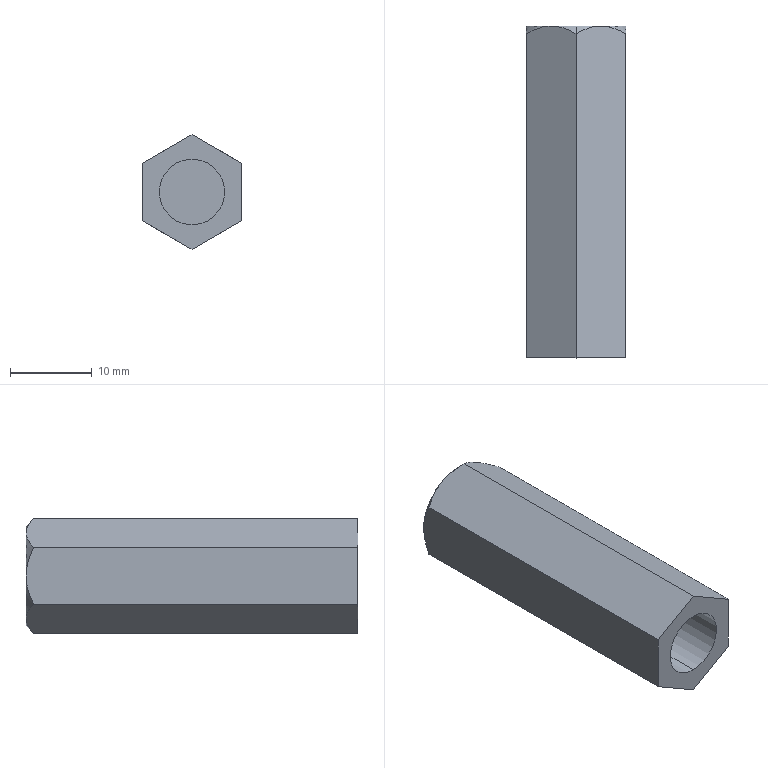Part | SolidWorks | features ICE 3, Extrusion 1 | 1 solid | 21 faces | box 12.124 x 40.5 x 14 mm | volume 4147 mm3 | plane 10 | cone 7 | cylinder 4 | commonest cylinder face diameters 8 x4
STEP:
#1=CARTESIAN_POINT('',(0.,10.,4.));
#2=VERTEX_POINT('',#1);
#3=CARTESIAN_POINT('',(0.,10.,-4.));
#4=VERTEX_POINT('',#3);
#5=CARTESIAN_POINT('',(0.,10.,0.));
#6=DIRECTION('',(0.,-1.,0.));
#7=DIRECTION('',(0.,0.,-1.));
#8=AXIS2_PLACEMENT_3D('',#5,#6,#7);
#9=CIRCLE('',#8,4.);
#10=EDGE_CURVE('',#2,#4,#9,.T.);
#11=ORIENTED_EDGE('',*,*,#10,.F.);
#12=CARTESIAN_POINT('',(0.,0.,4.));
#13=VERTEX_POINT('',#12);
#14=CARTESIAN_POINT('',(0.,10.,4.));
#15=DIRECTION('',(0.,-1.,0.));
#16=VECTOR('',#15,1000.);
#17=LINE('',#14,#16);
#18=EDGE_CURVE('',#2,#13,#17,.T.);
#19=ORIENTED_EDGE('',*,*,#18,.T.);
#20=CARTESIAN_POINT('',(0.,0.,-4.));
#21=VERTEX_POINT('',#20);
#22=CARTESIAN_POINT('',(0.,0.,0.));
#23=DIRECTION('',(0.,-1.,0.));
#24=DIRECTION('',(0.,0.,-1.));
#25=AXIS2_PLACEMENT_3D('',#22,#23,#24);
#26=CIRCLE('',#25,4.);
#27=EDGE_CURVE('',#13,#21,#26,.T.);
#28=ORIENTED_EDGE('',*,*,#27,.T.);
#29=CARTESIAN_POINT('',(0.,10.,-4.));
#30=DIRECTION('',(0.,-1.,0.));
#31=VECTOR('',#30,1000.);
#32=LINE('',#29,#31);
#33=EDGE_CURVE('',#4,#21,#32,.T.);
#34=ORIENTED_EDGE('',*,*,#33,.F.);
#35=EDGE_LOOP('',(#11,#19,#28,#34));
#36=FACE_OUTER_BOUND('',#35,.T.);
#37=CARTESIAN_POINT('',(0.,10.,0.));
#38=DIRECTION('',(0.,-1.,0.));
#39=DIRECTION('',(0.,0.,-1.));
#40=AXIS2_PLACEMENT_3D('',#37,#38,#39);
#41=CYLINDRICAL_SURFACE('',#40,4.);
#42=ADVANCED_FACE('',(#36),#41,.F.);
#43=CARTESIAN_POINT('',(0.,30.5,-4.));
#44=VERTEX_POINT('',#43);
#45=CARTESIAN_POINT('',(0.,30.5,4.));
#46=VERTEX_POINT('',#45);
#47=CARTESIAN_POINT('',(0.,30.5,0.));
#48=DIRECTION('',(0.,1.,0.));
#49=DIRECTION('',(0.,0.,1.));
#50=AXIS2_PLACEMENT_3D('',#47,#48,#49);
#51=CIRCLE('',#50,4.);
#52=EDGE_CURVE('',#44,#46,#51,.T.);
#53=ORIENTED_EDGE('',*,*,#52,.F.);
#54=CARTESIAN_POINT('',(0.,40.5,-4.));
#55=VERTEX_POINT('',#54);
#56=CARTESIAN_POINT('',(0.,30.5,-4.));
#57=DIRECTION('',(0.,1.,0.));
#58=VECTOR('',#57,1000.);
#59=LINE('',#56,#58);
#60=EDGE_CURVE('',#44,#55,#59,.T.);
#61=ORIENTED_EDGE('',*,*,#60,.T.);
#62=CARTESIAN_POINT('',(0.,40.5,4.));
#63=VERTEX_POINT('',#62);
#64=CARTESIAN_POINT('',(0.,40.5,0.));
#65=DIRECTION('',(0.,1.,0.));
#66=DIRECTION('',(0.,0.,1.));
#67=AXIS2_PLACEMENT_3D('',#64,#65,#66);
#68=CIRCLE('',#67,4.);
#69=EDGE_CURVE('',#55,#63,#68,.T.);
#70=ORIENTED_EDGE('',*,*,#69,.T.);
#71=CARTESIAN_POINT('',(0.,30.5,4.));
#72=DIRECTION('',(0.,1.,0.));
#73=VECTOR('',#72,1000.);
#74=LINE('',#71,#73);
#75=EDGE_CURVE('',#46,#63,#74,.T.);
#76=ORIENTED_EDGE('',*,*,#75,.F.);
#77=EDGE_LOOP('',(#53,#61,#70,#76));
#78=FACE_OUTER_BOUND('',#77,.T.);
#79=CARTESIAN_POINT('',(0.,30.5,0.));
#80=DIRECTION('',(0.,1.,0.));
#81=DIRECTION('',(0.,0.,1.));
#82=AXIS2_PLACEMENT_3D('',#79,#80,#81);
#83=CYLINDRICAL_SURFACE('',#82,4.);
#84=ADVANCED_FACE('',(#78),#83,.F.);
#85=CARTESIAN_POINT('',(0.,40.5,6.062));
#86=VERTEX_POINT('',#85);
#87=CARTESIAN_POINT('',(3.031,40.5,5.25));
#88=VERTEX_POINT('',#87);
#89=CARTESIAN_POINT('',(0.,40.5,0.));
#90=DIRECTION('',(0.,1.,0.));
#91=DIRECTION('',(0.,0.,1.));
#92=AXIS2_PLACEMENT_3D('',#89,#90,#91);
#93=CIRCLE('',#92,6.062);
#94=EDGE_CURVE('',#86,#88,#93,.T.);
#95=ORIENTED_EDGE('',*,*,#94,.F.);
#96=CARTESIAN_POINT('',(0.,39.562,7.));
#97=VERTEX_POINT('',#96);
#98=CARTESIAN_POINT('',(0.,40.5,6.062));
#99=DIRECTION('',(0.,-0.7071,0.7071));
#100=VECTOR('',#99,1000.);
#101=LINE('',#98,#100);
#102=EDGE_CURVE('',#86,#97,#101,.T.);
#103=ORIENTED_EDGE('',*,*,#102,.T.);
#104=CARTESIAN_POINT('',(3.031,40.5,5.25));
#105=CARTESIAN_POINT('',(2.504,40.5,5.554));
#106=CARTESIAN_POINT('',(1.986,40.407,5.854));
#107=CARTESIAN_POINT('',(0.9635,40.071,6.444));
#108=CARTESIAN_POINT('',(0.4748,39.836,6.726));
#109=CARTESIAN_POINT('',(0.,39.562,7.));
#110=B_SPLINE_CURVE_WITH_KNOTS('',3,(#104,#105,#106,#107,#108,#109),.UNSPECIFIED.,.F.,.F.,(4,2,4),(0.003628,0.00543,0.007231),.UNSPECIFIED.);
#111=EDGE_CURVE('',#88,#97,#110,.T.);
#112=ORIENTED_EDGE('',*,*,#111,.F.);
#113=EDGE_LOOP('',(#95,#103,#112));
#114=FACE_OUTER_BOUND('',#113,.T.);
#115=CARTESIAN_POINT('',(0.,40.5,0.));
#116=DIRECTION('',(0.,-1.,0.));
#117=DIRECTION('',(0.,0.,1.));
#118=AXIS2_PLACEMENT_3D('',#115,#116,#117);
#119=CONICAL_SURFACE('',#118,6.062,0.7854);
#120=ADVANCED_FACE('',(#114),#119,.T.);
#121=CARTESIAN_POINT('',(0.,39.562,-7.));
#122=VERTEX_POINT('',#121);
#123=CARTESIAN_POINT('',(3.031,40.5,-5.25));
#124=VERTEX_POINT('',#123);
#125=CARTESIAN_POINT('',(0.,39.562,-7.));
#126=CARTESIAN_POINT('',(0.4753,39.837,-6.726));
#127=CARTESIAN_POINT('',(0.9614,40.07,-6.445));
#128=CARTESIAN_POINT('',(1.717,40.319,-6.009));
#129=CARTESIAN_POINT('',(1.973,40.385,-5.861));
#130=CARTESIAN_POINT('',(2.496,40.476,-5.559));
#131=CARTESIAN_POINT('',(2.766,40.5,-5.403));
#132=CARTESIAN_POINT('',(3.031,40.5,-5.25));
#133=B_SPLINE_CURVE_WITH_KNOTS('',3,(#125,#126,#127,#128,#129,#130,#131,#132),.UNSPECIFIED.,.F.,.F.,(4,2,2,4),(0.000000254,0.001814,0.002721,0.003628),.UNSPECIFIED.);
#134=EDGE_CURVE('',#122,#124,#133,.T.);
#135=ORIENTED_EDGE('',*,*,#134,.T.);
#136=CARTESIAN_POINT('',(6.062,39.562,-3.5));
#137=VERTEX_POINT('',#136);
#138=CARTESIAN_POINT('',(3.031,40.5,-5.25));
#139=CARTESIAN_POINT('',(3.558,40.5,-4.946));
#140=CARTESIAN_POINT('',(4.077,40.407,-4.646));
#141=CARTESIAN_POINT('',(5.099,40.071,-4.056));
#142=CARTESIAN_POINT('',(5.587,39.836,-3.774));
#143=CARTESIAN_POINT('',(6.062,39.562,-3.5));
#144=B_SPLINE_CURVE_WITH_KNOTS('',3,(#138,#139,#140,#141,#142,#143),.UNSPECIFIED.,.F.,.F.,(4,2,4),(0.003628,0.00543,0.007231),.UNSPECIFIED.);
#145=EDGE_CURVE('',#124,#137,#144,.T.);
#146=ORIENTED_EDGE('',*,*,#145,.T.);
#147=CARTESIAN_POINT('',(6.062,0.,-3.5));
#148=VERTEX_POINT('',#147);
#149=CARTESIAN_POINT('',(6.062,40.5,-3.5));
#150=DIRECTION('',(0.,-1.,0.));
#151=VECTOR('',#150,1000.);
#152=LINE('',#149,#151);
#153=EDGE_CURVE('',#137,#148,#152,.T.);
#154=ORIENTED_EDGE('',*,*,#153,.T.);
#155=CARTESIAN_POINT('',(0.,0.,-7.));
#156=VERTEX_POINT('',#155);
#157=CARTESIAN_POINT('',(6.062,0.,-3.5));
#158=DIRECTION('',(-0.866,0.,-0.5));
#159=VECTOR('',#158,1000.);
#160=LINE('',#157,#159);
#161=EDGE_CURVE('',#148,#156,#160,.T.);
#162=ORIENTED_EDGE('',*,*,#161,.T.);
#163=CARTESIAN_POINT('',(0.,40.5,-7.));
#164=DIRECTION('',(0.,-1.,0.));
#165=VECTOR('',#164,1000.);
#166=LINE('',#163,#165);
#167=EDGE_CURVE('',#122,#156,#166,.T.);
#168=ORIENTED_EDGE('',*,*,#167,.F.);
#169=EDGE_LOOP('',(#135,#146,#154,#162,#168));
#170=FACE_OUTER_BOUND('',#169,.T.);
#171=CARTESIAN_POINT('',(6.062,40.5,-3.5));
#172=DIRECTION('',(-0.5,0.,0.866));
#173=DIRECTION('',(0.866,0.,0.5));
#174=AXIS2_PLACEMENT_3D('',#171,#172,#173);
#175=PLANE('',#174);
#176=ADVANCED_FACE('',(#170),#175,.F.);
#177=CARTESIAN_POINT('',(-6.062,39.562,-3.5));
#178=VERTEX_POINT('',#177);
#179=CARTESIAN_POINT('',(-3.031,40.5,-5.25));
#180=VERTEX_POINT('',#179);
#181=CARTESIAN_POINT('',(-6.062,39.562,-3.5));
#182=CARTESIAN_POINT('',(-5.587,39.837,-3.774));
#183=CARTESIAN_POINT('',(-5.101,40.07,-4.055));
#184=CARTESIAN_POINT('',(-4.345,40.319,-4.491));
#185=CARTESIAN_POINT('',(-4.089,40.385,-4.639));
#186=CARTESIAN_POINT('',(-3.566,40.476,-4.941));
#187=CARTESIAN_POINT('',(-3.297,40.5,-5.097));
#188=CARTESIAN_POINT('',(-3.031,40.5,-5.25));
#189=B_SPLINE_CURVE_WITH_KNOTS('',3,(#181,#182,#183,#184,#185,#186,#187,#188),.UNSPECIFIED.,.F.,.F.,(4,2,2,4),(0.000000254,0.001814,0.002721,0.003628),.UNSPECIFIED.);
#190=EDGE_CURVE('',#178,#180,#189,.T.);
#191=ORIENTED_EDGE('',*,*,#190,.T.);
#192=CARTESIAN_POINT('',(-3.031,40.5,-5.25));
#193=CARTESIAN_POINT('',(-2.504,40.5,-5.554));
#194=CARTESIAN_POINT('',(-1.986,40.407,-5.854));
#195=CARTESIAN_POINT('',(-0.9635,40.071,-6.444));
#196=CARTESIAN_POINT('',(-0.4748,39.836,-6.726));
#197=CARTESIAN_POINT('',(0.,39.562,-7.));
#198=B_SPLINE_CURVE_WITH_KNOTS('',3,(#192,#193,#194,#195,#196,#197),.UNSPECIFIED.,.F.,.F.,(4,2,4),(0.003628,0.00543,0.007231),.UNSPECIFIED.);
#199=EDGE_CURVE('',#180,#122,#198,.T.);
#200=ORIENTED_EDGE('',*,*,#199,.T.);
#201=ORIENTED_EDGE('',*,*,#167,.T.);
#202=CARTESIAN_POINT('',(-6.062,0.,-3.5));
#203=VERTEX_POINT('',#202);
#204=CARTESIAN_POINT('',(0.,0.,-7.));
#205=DIRECTION('',(-0.866,0.,0.5));
#206=VECTOR('',#205,1000.);
#207=LINE('',#204,#206);
#208=EDGE_CURVE('',#156,#203,#207,.T.);
#209=ORIENTED_EDGE('',*,*,#208,.T.);
#210=CARTESIAN_POINT('',(-6.062,40.5,-3.5));
#211=DIRECTION('',(0.,-1.,0.));
#212=VECTOR('',#211,1000.);
#213=LINE('',#210,#212);
#214=EDGE_CURVE('',#178,#203,#213,.T.);
#215=ORIENTED_EDGE('',*,*,#214,.F.);
#216=EDGE_LOOP('',(#191,#200,#201,#209,#215));
#217=FACE_OUTER_BOUND('',#216,.T.);
#218=CARTESIAN_POINT('',(0.,40.5,-7.));
#219=DIRECTION('',(0.5,0.,0.866));
#220=DIRECTION('',(0.866,0.,-0.5));
#221=AXIS2_PLACEMENT_3D('',#218,#219,#220);
#222=PLANE('',#221);
#223=ADVANCED_FACE('',(#217),#222,.F.);
#224=CARTESIAN_POINT('',(-6.062,39.562,3.5));
#225=VERTEX_POINT('',#224);
#226=CARTESIAN_POINT('',(-6.062,40.5,0.));
#227=VERTEX_POINT('',#226);
#228=CARTESIAN_POINT('',(-6.062,39.562,3.5));
#229=CARTESIAN_POINT('',(-6.062,39.698,3.229));
#230=CARTESIAN_POINT('',(-6.062,39.824,2.954));
#231=CARTESIAN_POINT('',(-6.062,40.051,2.389));
#232=CARTESIAN_POINT('',(-6.062,40.154,2.098));
#233=CARTESIAN_POINT('',(-6.062,40.405,1.215));
#234=CARTESIAN_POINT('',(-6.062,40.5,0.6148));
#235=CARTESIAN_POINT('',(-6.062,40.5,0.));
#236=B_SPLINE_CURVE_WITH_KNOTS('',3,(#228,#229,#230,#231,#232,#233,#234,#235),.UNSPECIFIED.,.F.,.F.,(4,2,2,4),(0.02356,0.02447,0.02537,0.02719),.UNSPECIFIED.);
#237=EDGE_CURVE('',#225,#227,#236,.T.);
#238=ORIENTED_EDGE('',*,*,#237,.T.);
#239=CARTESIAN_POINT('',(-6.062,40.5,0.));
#240=CARTESIAN_POINT('',(-6.062,40.5,-0.3069));
#241=CARTESIAN_POINT('',(-6.062,40.476,-0.6142));
#242=CARTESIAN_POINT('',(-6.062,40.386,-1.217));
#243=CARTESIAN_POINT('',(-6.062,40.32,-1.515));
#244=CARTESIAN_POINT('',(-6.062,40.151,-2.105));
#245=CARTESIAN_POINT('',(-6.062,40.049,-2.395));
#246=CARTESIAN_POINT('',(-6.062,39.822,-2.957));
#247=CARTESIAN_POINT('',(-6.062,39.697,-3.231));
#248=CARTESIAN_POINT('',(-6.062,39.562,-3.5));
#249=B_SPLINE_CURVE_WITH_KNOTS('',3,(#239,#240,#241,#242,#243,#244,#245,#246,#247,#248),.UNSPECIFIED.,.F.,.F.,(4,2,2,2,4),(0.02719,0.0281,0.029,0.02991,0.03082),.UNSPECIFIED.);
#250=EDGE_CURVE('',#227,#178,#249,.T.);
#251=ORIENTED_EDGE('',*,*,#250,.T.);
#252=ORIENTED_EDGE('',*,*,#214,.T.);
#253=CARTESIAN_POINT('',(-6.062,0.,3.5));
#254=VERTEX_POINT('',#253);
#255=CARTESIAN_POINT('',(-6.062,0.,-3.5));
#256=DIRECTION('',(0.,0.,1.));
#257=VECTOR('',#256,1000.);
#258=LINE('',#255,#257);
#259=EDGE_CURVE('',#203,#254,#258,.T.);
#260=ORIENTED_EDGE('',*,*,#259,.T.);
#261=CARTESIAN_POINT('',(-6.062,40.5,3.5));
#262=DIRECTION('',(0.,-1.,0.));
#263=VECTOR('',#262,1000.);
#264=LINE('',#261,#263);
#265=EDGE_CURVE('',#225,#254,#264,.T.);
#266=ORIENTED_EDGE('',*,*,#265,.F.);
#267=EDGE_LOOP('',(#238,#251,#252,#260,#266));
#268=FACE_OUTER_BOUND('',#267,.T.);
#269=CARTESIAN_POINT('',(-6.062,40.5,-3.5));
#270=DIRECTION('',(1.,0.,0.));
#271=DIRECTION('',(0.,0.,-1.));
#272=AXIS2_PLACEMENT_3D('',#269,#270,#271);
#273=PLANE('',#272);
#274=ADVANCED_FACE('',(#268),#273,.F.);
#275=CARTESIAN_POINT('',(-3.031,40.5,5.25));
#276=VERTEX_POINT('',#275);
#277=CARTESIAN_POINT('',(-3.031,40.5,5.25));
#278=CARTESIAN_POINT('',(-3.558,40.5,4.946));
#279=CARTESIAN_POINT('',(-4.077,40.407,4.646));
#280=CARTESIAN_POINT('',(-5.099,40.071,4.056));
#281=CARTESIAN_POINT('',(-5.587,39.836,3.774));
#282=CARTESIAN_POINT('',(-6.062,39.562,3.5));
#283=B_SPLINE_CURVE_WITH_KNOTS('',3,(#277,#278,#279,#280,#281,#282),.UNSPECIFIED.,.F.,.F.,(4,2,4),(0.003628,0.00543,0.007231),.UNSPECIFIED.);
#284=EDGE_CURVE('',#276,#225,#283,.T.);
#285=ORIENTED_EDGE('',*,*,#284,.T.);
#286=ORIENTED_EDGE('',*,*,#265,.T.);
#287=CARTESIAN_POINT('',(0.,0.,7.));
#288=VERTEX_POINT('',#287);
#289=CARTESIAN_POINT('',(-6.062,0.,3.5));
#290=DIRECTION('',(0.866,0.,0.5));
#291=VECTOR('',#290,1000.);
#292=LINE('',#289,#291);
#293=EDGE_CURVE('',#254,#288,#292,.T.);
#294=ORIENTED_EDGE('',*,*,#293,.T.);
#295=CARTESIAN_POINT('',(0.,40.5,7.));
#296=DIRECTION('',(0.,-1.,0.));
#297=VECTOR('',#296,1000.);
#298=LINE('',#295,#297);
#299=EDGE_CURVE('',#97,#288,#298,.T.);
#300=ORIENTED_EDGE('',*,*,#299,.F.);
#301=CARTESIAN_POINT('',(0.,39.562,7.));
#302=CARTESIAN_POINT('',(-0.4753,39.837,6.726));
#303=CARTESIAN_POINT('',(-0.9614,40.07,6.445));
#304=CARTESIAN_POINT('',(-1.717,40.319,6.009));
#305=CARTESIAN_POINT('',(-1.973,40.385,5.861));
#306=CARTESIAN_POINT('',(-2.496,40.476,5.559));
#307=CARTESIAN_POINT('',(-2.766,40.5,5.403));
#308=CARTESIAN_POINT('',(-3.031,40.5,5.25));
#309=B_SPLINE_CURVE_WITH_KNOTS('',3,(#301,#302,#303,#304,#305,#306,#307,#308),.UNSPECIFIED.,.F.,.F.,(4,2,2,4),(0.000000254,0.001814,0.002721,0.003628),.UNSPECIFIED.);
#310=EDGE_CURVE('',#97,#276,#309,.T.);
#311=ORIENTED_EDGE('',*,*,#310,.T.);
#312=EDGE_LOOP('',(#285,#286,#294,#300,#311));
#313=FACE_OUTER_BOUND('',#312,.T.);
#314=CARTESIAN_POINT('',(-6.062,40.5,3.5));
#315=DIRECTION('',(0.5,0.,-0.866));
#316=DIRECTION('',(-0.866,0.,-0.5));
#317=AXIS2_PLACEMENT_3D('',#314,#315,#316);
#318=PLANE('',#317);
#319=ADVANCED_FACE('',(#313),#318,.F.);
#320=ORIENTED_EDGE('',*,*,#111,.T.);
#321=ORIENTED_EDGE('',*,*,#299,.T.);
#322=CARTESIAN_POINT('',(6.062,0.,3.5));
#323=VERTEX_POINT('',#322);
#324=CARTESIAN_POINT('',(0.,0.,7.));
#325=DIRECTION('',(0.866,0.,-0.5));
#326=VECTOR('',#325,1000.);
#327=LINE('',#324,#326);
#328=EDGE_CURVE('',#288,#323,#327,.T.);
#329=ORIENTED_EDGE('',*,*,#328,.T.);
#330=CARTESIAN_POINT('',(6.062,39.562,3.5));
#331=VERTEX_POINT('',#330);
#332=CARTESIAN_POINT('',(6.062,40.5,3.5));
#333=DIRECTION('',(0.,-1.,0.));
#334=VECTOR('',#333,1000.);
#335=LINE('',#332,#334);
#336=EDGE_CURVE('',#331,#323,#335,.T.);
#337=ORIENTED_EDGE('',*,*,#336,.F.);
#338=CARTESIAN_POINT('',(6.062,39.562,3.5));
#339=CARTESIAN_POINT('',(5.587,39.837,3.774));
#340=CARTESIAN_POINT('',(5.101,40.07,4.055));
#341=CARTESIAN_POINT('',(4.345,40.319,4.491));
#342=CARTESIAN_POINT('',(4.089,40.385,4.639));
#343=CARTESIAN_POINT('',(3.566,40.476,4.941));
#344=CARTESIAN_POINT('',(3.297,40.5,5.097));
#345=CARTESIAN_POINT('',(3.031,40.5,5.25));
#346=B_SPLINE_CURVE_WITH_KNOTS('',3,(#338,#339,#340,#341,#342,#343,#344,#345),.UNSPECIFIED.,.F.,.F.,(4,2,2,4),(0.000000254,0.001814,0.002721,0.003628),.UNSPECIFIED.);
#347=EDGE_CURVE('',#331,#88,#346,.T.);
#348=ORIENTED_EDGE('',*,*,#347,.T.);
#349=EDGE_LOOP('',(#320,#321,#329,#337,#348));
#350=FACE_OUTER_BOUND('',#349,.T.);
#351=CARTESIAN_POINT('',(0.,40.5,7.));
#352=DIRECTION('',(-0.5,0.,-0.866));
#353=DIRECTION('',(-0.866,0.,0.5));
#354=AXIS2_PLACEMENT_3D('',#351,#352,#353);
#355=PLANE('',#354);
#356=ADVANCED_FACE('',(#350),#355,.F.);
#357=CARTESIAN_POINT('',(6.062,40.5,0.));
#358=VERTEX_POINT('',#357);
#359=CARTESIAN_POINT('',(6.062,39.562,-3.5));
#360=CARTESIAN_POINT('',(6.062,39.697,-3.231));
#361=CARTESIAN_POINT('',(6.062,39.822,-2.957));
#362=CARTESIAN_POINT('',(6.062,40.049,-2.395));
#363=CARTESIAN_POINT('',(6.062,40.151,-2.105));
#364=CARTESIAN_POINT('',(6.062,40.32,-1.515));
#365=CARTESIAN_POINT('',(6.062,40.386,-1.217));
#366=CARTESIAN_POINT('',(6.062,40.476,-0.6142));
#367=CARTESIAN_POINT('',(6.062,40.5,-0.3069));
#368=CARTESIAN_POINT('',(6.062,40.5,0.));
#369=B_SPLINE_CURVE_WITH_KNOTS('',3,(#359,#360,#361,#362,#363,#364,#365,#366,#367,#368),.UNSPECIFIED.,.F.,.F.,(4,2,2,2,4),(0.02208,0.02298,0.02388,0.02479,0.02569),.UNSPECIFIED.);
#370=EDGE_CURVE('',#137,#358,#369,.T.);
#371=ORIENTED_EDGE('',*,*,#370,.T.);
#372=CARTESIAN_POINT('',(6.062,40.5,0.));
#373=CARTESIAN_POINT('',(6.062,40.5,0.6148));
#374=CARTESIAN_POINT('',(6.062,40.405,1.215));
#375=CARTESIAN_POINT('',(6.062,40.154,2.098));
#376=CARTESIAN_POINT('',(6.062,40.051,2.389));
#377=CARTESIAN_POINT('',(6.062,39.824,2.954));
#378=CARTESIAN_POINT('',(6.062,39.698,3.229));
#379=CARTESIAN_POINT('',(6.062,39.562,3.5));
#380=B_SPLINE_CURVE_WITH_KNOTS('',3,(#372,#373,#374,#375,#376,#377,#378,#379),.UNSPECIFIED.,.F.,.F.,(4,2,2,4),(0.02569,0.0275,0.02841,0.02931),.UNSPECIFIED.);
#381=EDGE_CURVE('',#358,#331,#380,.T.);
#382=ORIENTED_EDGE('',*,*,#381,.T.);
#383=ORIENTED_EDGE('',*,*,#336,.T.);
#384=CARTESIAN_POINT('',(6.062,0.,3.5));
#385=DIRECTION('',(0.,0.,-1.));
#386=VECTOR('',#385,1000.);
#387=LINE('',#384,#386);
#388=EDGE_CURVE('',#323,#148,#387,.T.);
#389=ORIENTED_EDGE('',*,*,#388,.T.);
#390=ORIENTED_EDGE('',*,*,#153,.F.);
#391=EDGE_LOOP('',(#371,#382,#383,#389,#390));
#392=FACE_OUTER_BOUND('',#391,.T.);
#393=CARTESIAN_POINT('',(6.062,40.5,3.5));
#394=DIRECTION('',(-1.,0.,0.));
#395=DIRECTION('',(0.,0.,1.));
#396=AXIS2_PLACEMENT_3D('',#393,#394,#395);
#397=PLANE('',#396);
#398=ADVANCED_FACE('',(#392),#397,.F.);
#399=CARTESIAN_POINT('',(0.,0.,0.));
#400=DIRECTION('',(0.,-1.,0.));
#401=DIRECTION('',(0.,0.,-1.));
#402=AXIS2_PLACEMENT_3D('',#399,#400,#401);
#403=CIRCLE('',#402,4.);
#404=EDGE_CURVE('',#21,#13,#403,.T.);
#405=ORIENTED_EDGE('',*,*,#404,.F.);
#406=ORIENTED_EDGE('',*,*,#27,.F.);
#407=EDGE_LOOP('',(#405,#406));
#408=FACE_BOUND('',#407,.T.);
#409=ORIENTED_EDGE('',*,*,#161,.F.);
#410=ORIENTED_EDGE('',*,*,#388,.F.);
#411=ORIENTED_EDGE('',*,*,#328,.F.);
#412=ORIENTED_EDGE('',*,*,#293,.F.);
#413=ORIENTED_EDGE('',*,*,#259,.F.);
#414=ORIENTED_EDGE('',*,*,#208,.F.);
#415=EDGE_LOOP('',(#409,#410,#411,#412,#413,#414));
#416=FACE_OUTER_BOUND('',#415,.T.);
#417=CARTESIAN_POINT('',(0.,0.,0.));
#418=DIRECTION('',(0.,1.,0.));
#419=DIRECTION('',(0.,0.,1.));
#420=AXIS2_PLACEMENT_3D('',#417,#418,#419);
#421=PLANE('',#420);
#422=ADVANCED_FACE('',(#408,#416),#421,.F.);
#423=ORIENTED_EDGE('',*,*,#347,.F.);
#424=ORIENTED_EDGE('',*,*,#381,.F.);
#425=CARTESIAN_POINT('',(0.,40.5,0.));
#426=DIRECTION('',(0.,1.,0.));
#427=DIRECTION('',(0.,0.,1.));
#428=AXIS2_PLACEMENT_3D('',#425,#426,#427);
#429=CIRCLE('',#428,6.062);
#430=EDGE_CURVE('',#88,#358,#429,.T.);
#431=ORIENTED_EDGE('',*,*,#430,.F.);
#432=EDGE_LOOP('',(#423,#424,#431));
#433=FACE_OUTER_BOUND('',#432,.T.);
#434=CARTESIAN_POINT('',(0.,40.5,0.));
#435=DIRECTION('',(0.,-1.,0.));
#436=DIRECTION('',(0.,0.,1.));
#437=AXIS2_PLACEMENT_3D('',#434,#435,#436);
#438=CONICAL_SURFACE('',#437,6.062,0.7854);
#439=ADVANCED_FACE('',(#433),#438,.T.);
#440=ORIENTED_EDGE('',*,*,#145,.F.);
#441=CARTESIAN_POINT('',(0.,40.5,0.));
#442=DIRECTION('',(0.,1.,0.));
#443=DIRECTION('',(0.,0.,1.));
#444=AXIS2_PLACEMENT_3D('',#441,#442,#443);
#445=CIRCLE('',#444,6.062);
#446=EDGE_CURVE('',#358,#124,#445,.T.);
#447=ORIENTED_EDGE('',*,*,#446,.F.);
#448=ORIENTED_EDGE('',*,*,#370,.F.);
#449=EDGE_LOOP('',(#440,#447,#448));
#450=FACE_OUTER_BOUND('',#449,.T.);
#451=CARTESIAN_POINT('',(0.,40.5,0.));
#452=DIRECTION('',(0.,-1.,0.));
#453=DIRECTION('',(0.,0.,1.));
#454=AXIS2_PLACEMENT_3D('',#451,#452,#453);
#455=CONICAL_SURFACE('',#454,6.062,0.7854);
#456=ADVANCED_FACE('',(#450),#455,.T.);
#457=ORIENTED_EDGE('',*,*,#102,.F.);
#458=CARTESIAN_POINT('',(0.,40.5,0.));
#459=DIRECTION('',(0.,1.,0.));
#460=DIRECTION('',(0.,0.,1.));
#461=AXIS2_PLACEMENT_3D('',#458,#459,#460);
#462=CIRCLE('',#461,6.062);
#463=EDGE_CURVE('',#276,#86,#462,.T.);
#464=ORIENTED_EDGE('',*,*,#463,.F.);
#465=ORIENTED_EDGE('',*,*,#310,.F.);
#466=EDGE_LOOP('',(#457,#464,#465));
#467=FACE_OUTER_BOUND('',#466,.T.);
#468=CARTESIAN_POINT('',(0.,40.5,0.));
#469=DIRECTION('',(0.,-1.,0.));
#470=DIRECTION('',(0.,0.,1.));
#471=AXIS2_PLACEMENT_3D('',#468,#469,#470);
#472=CONICAL_SURFACE('',#471,6.062,0.7854);
#473=ADVANCED_FACE('',(#467),#472,.T.);
#474=ORIENTED_EDGE('',*,*,#199,.F.);
#475=CARTESIAN_POINT('',(0.,40.5,0.));
#476=DIRECTION('',(0.,1.,0.));
#477=DIRECTION('',(0.,0.,1.));
#478=AXIS2_PLACEMENT_3D('',#475,#476,#477);
#479=CIRCLE('',#478,6.062);
#480=EDGE_CURVE('',#124,#180,#479,.T.);
#481=ORIENTED_EDGE('',*,*,#480,.F.);
#482=ORIENTED_EDGE('',*,*,#134,.F.);
#483=EDGE_LOOP('',(#474,#481,#482));
#484=FACE_OUTER_BOUND('',#483,.T.);
#485=CARTESIAN_POINT('',(0.,40.5,0.));
#486=DIRECTION('',(0.,-1.,0.));
#487=DIRECTION('',(0.,0.,1.));
#488=AXIS2_PLACEMENT_3D('',#485,#486,#487);
#489=CONICAL_SURFACE('',#488,6.062,0.7854);
#490=ADVANCED_FACE('',(#484),#489,.T.);
#491=ORIENTED_EDGE('',*,*,#250,.F.);
#492=CARTESIAN_POINT('',(0.,40.5,0.));
#493=DIRECTION('',(0.,1.,0.));
#494=DIRECTION('',(0.,0.,1.));
#495=AXIS2_PLACEMENT_3D('',#492,#493,#494);
#496=CIRCLE('',#495,6.062);
#497=EDGE_CURVE('',#180,#227,#496,.T.);
#498=ORIENTED_EDGE('',*,*,#497,.F.);
#499=ORIENTED_EDGE('',*,*,#190,.F.);
#500=EDGE_LOOP('',(#491,#498,#499));
#501=FACE_OUTER_BOUND('',#500,.T.);
#502=CARTESIAN_POINT('',(0.,40.5,0.));
#503=DIRECTION('',(0.,-1.,0.));
#504=DIRECTION('',(0.,0.,1.));
#505=AXIS2_PLACEMENT_3D('',#502,#503,#504);
#506=CONICAL_SURFACE('',#505,6.062,0.7854);
#507=ADVANCED_FACE('',(#501),#506,.T.);
#508=ORIENTED_EDGE('',*,*,#237,.F.);
#509=ORIENTED_EDGE('',*,*,#284,.F.);
#510=CARTESIAN_POINT('',(0.,40.5,0.));
#511=DIRECTION('',(0.,1.,0.));
#512=DIRECTION('',(0.,0.,1.));
#513=AXIS2_PLACEMENT_3D('',#510,#511,#512);
#514=CIRCLE('',#513,6.062);
#515=EDGE_CURVE('',#227,#276,#514,.T.);
#516=ORIENTED_EDGE('',*,*,#515,.F.);
#517=EDGE_LOOP('',(#508,#509,#516));
#518=FACE_OUTER_BOUND('',#517,.T.);
#519=CARTESIAN_POINT('',(0.,40.5,0.));
#520=DIRECTION('',(0.,-1.,0.));
#521=DIRECTION('',(0.,0.,1.));
#522=AXIS2_PLACEMENT_3D('',#519,#520,#521);
#523=CONICAL_SURFACE('',#522,6.062,0.7854);
#524=ADVANCED_FACE('',(#518),#523,.T.);
#525=CARTESIAN_POINT('',(0.,40.5,0.));
#526=DIRECTION('',(0.,1.,0.));
#527=DIRECTION('',(0.,0.,1.));
#528=AXIS2_PLACEMENT_3D('',#525,#526,#527);
#529=CIRCLE('',#528,4.);
#530=EDGE_CURVE('',#63,#55,#529,.T.);
#531=ORIENTED_EDGE('',*,*,#530,.F.);
#532=ORIENTED_EDGE('',*,*,#69,.F.);
#533=EDGE_LOOP('',(#531,#532));
#534=FACE_BOUND('',#533,.T.);
#535=ORIENTED_EDGE('',*,*,#497,.T.);
#536=ORIENTED_EDGE('',*,*,#515,.T.);
#537=ORIENTED_EDGE('',*,*,#463,.T.);
#538=ORIENTED_EDGE('',*,*,#94,.T.);
#539=ORIENTED_EDGE('',*,*,#430,.T.);
#540=ORIENTED_EDGE('',*,*,#446,.T.);
#541=ORIENTED_EDGE('',*,*,#480,.T.);
#542=EDGE_LOOP('',(#535,#536,#537,#538,#539,#540,#541));
#543=FACE_OUTER_BOUND('',#542,.T.);
#544=CARTESIAN_POINT('',(0.,40.5,0.));
#545=DIRECTION('',(0.,1.,0.));
#546=DIRECTION('',(0.,0.,1.));
#547=AXIS2_PLACEMENT_3D('',#544,#545,#546);
#548=PLANE('',#547);
#549=ADVANCED_FACE('',(#534,#543),#548,.T.);
#550=ORIENTED_EDGE('',*,*,#60,.F.);
#551=CARTESIAN_POINT('',(0.,30.5,0.));
#552=DIRECTION('',(0.,1.,0.));
#553=DIRECTION('',(0.,0.,1.));
#554=AXIS2_PLACEMENT_3D('',#551,#552,#553);
#555=CIRCLE('',#554,4.);
#556=EDGE_CURVE('',#46,#44,#555,.T.);
#557=ORIENTED_EDGE('',*,*,#556,.F.);
#558=ORIENTED_EDGE('',*,*,#75,.T.);
#559=ORIENTED_EDGE('',*,*,#530,.T.);
#560=EDGE_LOOP('',(#550,#557,#558,#559));
#561=FACE_OUTER_BOUND('',#560,.T.);
#562=CARTESIAN_POINT('',(0.,30.5,0.));
#563=DIRECTION('',(0.,1.,0.));
#564=DIRECTION('',(0.,0.,1.));
#565=AXIS2_PLACEMENT_3D('',#562,#563,#564);
#566=CYLINDRICAL_SURFACE('',#565,4.);
#567=ADVANCED_FACE('',(#561),#566,.F.);
#568=ORIENTED_EDGE('',*,*,#556,.T.);
#569=ORIENTED_EDGE('',*,*,#52,.T.);
#570=EDGE_LOOP('',(#568,#569));
#571=FACE_OUTER_BOUND('',#570,.T.);
#572=CARTESIAN_POINT('',(0.,30.5,0.));
#573=DIRECTION('',(0.,1.,0.));
#574=DIRECTION('',(0.,0.,1.));
#575=AXIS2_PLACEMENT_3D('',#572,#573,#574);
#576=PLANE('',#575);
#577=ADVANCED_FACE('',(#571),#576,.T.);
#578=ORIENTED_EDGE('',*,*,#18,.F.);
#579=CARTESIAN_POINT('',(0.,10.,0.));
#580=DIRECTION('',(0.,-1.,0.));
#581=DIRECTION('',(0.,0.,-1.));
#582=AXIS2_PLACEMENT_3D('',#579,#580,#581);
#583=CIRCLE('',#582,4.);
#584=EDGE_CURVE('',#4,#2,#583,.T.);
#585=ORIENTED_EDGE('',*,*,#584,.F.);
#586=ORIENTED_EDGE('',*,*,#33,.T.);
#587=ORIENTED_EDGE('',*,*,#404,.T.);
#588=EDGE_LOOP('',(#578,#585,#586,#587));
#589=FACE_OUTER_BOUND('',#588,.T.);
#590=CARTESIAN_POINT('',(0.,10.,0.));
#591=DIRECTION('',(0.,-1.,0.));
#592=DIRECTION('',(0.,0.,-1.));
#593=AXIS2_PLACEMENT_3D('',#590,#591,#592);
#594=CYLINDRICAL_SURFACE('',#593,4.);
#595=ADVANCED_FACE('',(#589),#594,.F.);
#596=ORIENTED_EDGE('',*,*,#584,.T.);
#597=ORIENTED_EDGE('',*,*,#10,.T.);
#598=EDGE_LOOP('',(#596,#597));
#599=FACE_OUTER_BOUND('',#598,.T.);
#600=CARTESIAN_POINT('',(0.,10.,0.));
#601=DIRECTION('',(0.,-1.,0.));
#602=DIRECTION('',(0.,0.,-1.));
#603=AXIS2_PLACEMENT_3D('',#600,#601,#602);
#604=PLANE('',#603);
#605=ADVANCED_FACE('',(#599),#604,.T.);
#606=CLOSED_SHELL('',(#42,#84,#120,#176,#223,#274,#319,#356,#398,#422,#439,#456,#473,#490,#507,#524,#549,#567,#577,#595,#605));
#607=MANIFOLD_SOLID_BREP('',#606);
#608=CARTESIAN_POINT('',(0.,0.,0.));
#609=DIRECTION('',(0.,0.,1.));
#610=DIRECTION('',(1.,0.,0.));
#611=AXIS2_PLACEMENT_3D('',#608,#609,#610);
#612=(LENGTH_UNIT()NAMED_UNIT(*)SI_UNIT(.MILLI.,.METRE.));
#613=UNCERTAINTY_MEASURE_WITH_UNIT(LENGTH_MEASURE(0.00001),#612,'','');
#614=(NAMED_UNIT(*)PLANE_ANGLE_UNIT()SI_UNIT($,.RADIAN.));
#615=(NAMED_UNIT(*)SI_UNIT($,.STERADIAN.)SOLID_ANGLE_UNIT());
#616=(GEOMETRIC_REPRESENTATION_CONTEXT(3)GLOBAL_UNCERTAINTY_ASSIGNED_CONTEXT((#613))GLOBAL_UNIT_ASSIGNED_CONTEXT((#612,#614,#615))REPRESENTATION_CONTEXT('',''));
#617=ADVANCED_BREP_SHAPE_REPRESENTATION('',(#607,#611),#616);